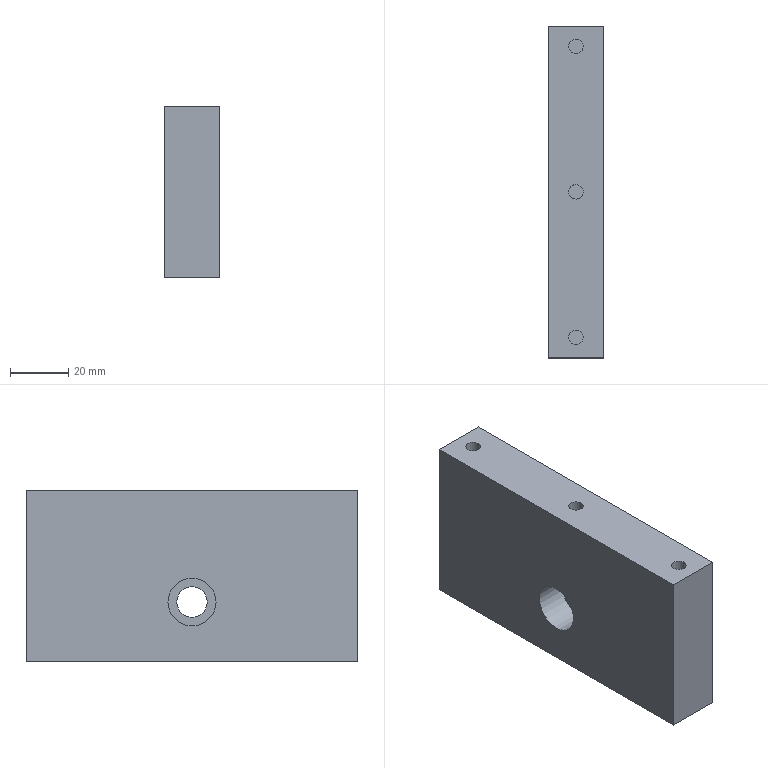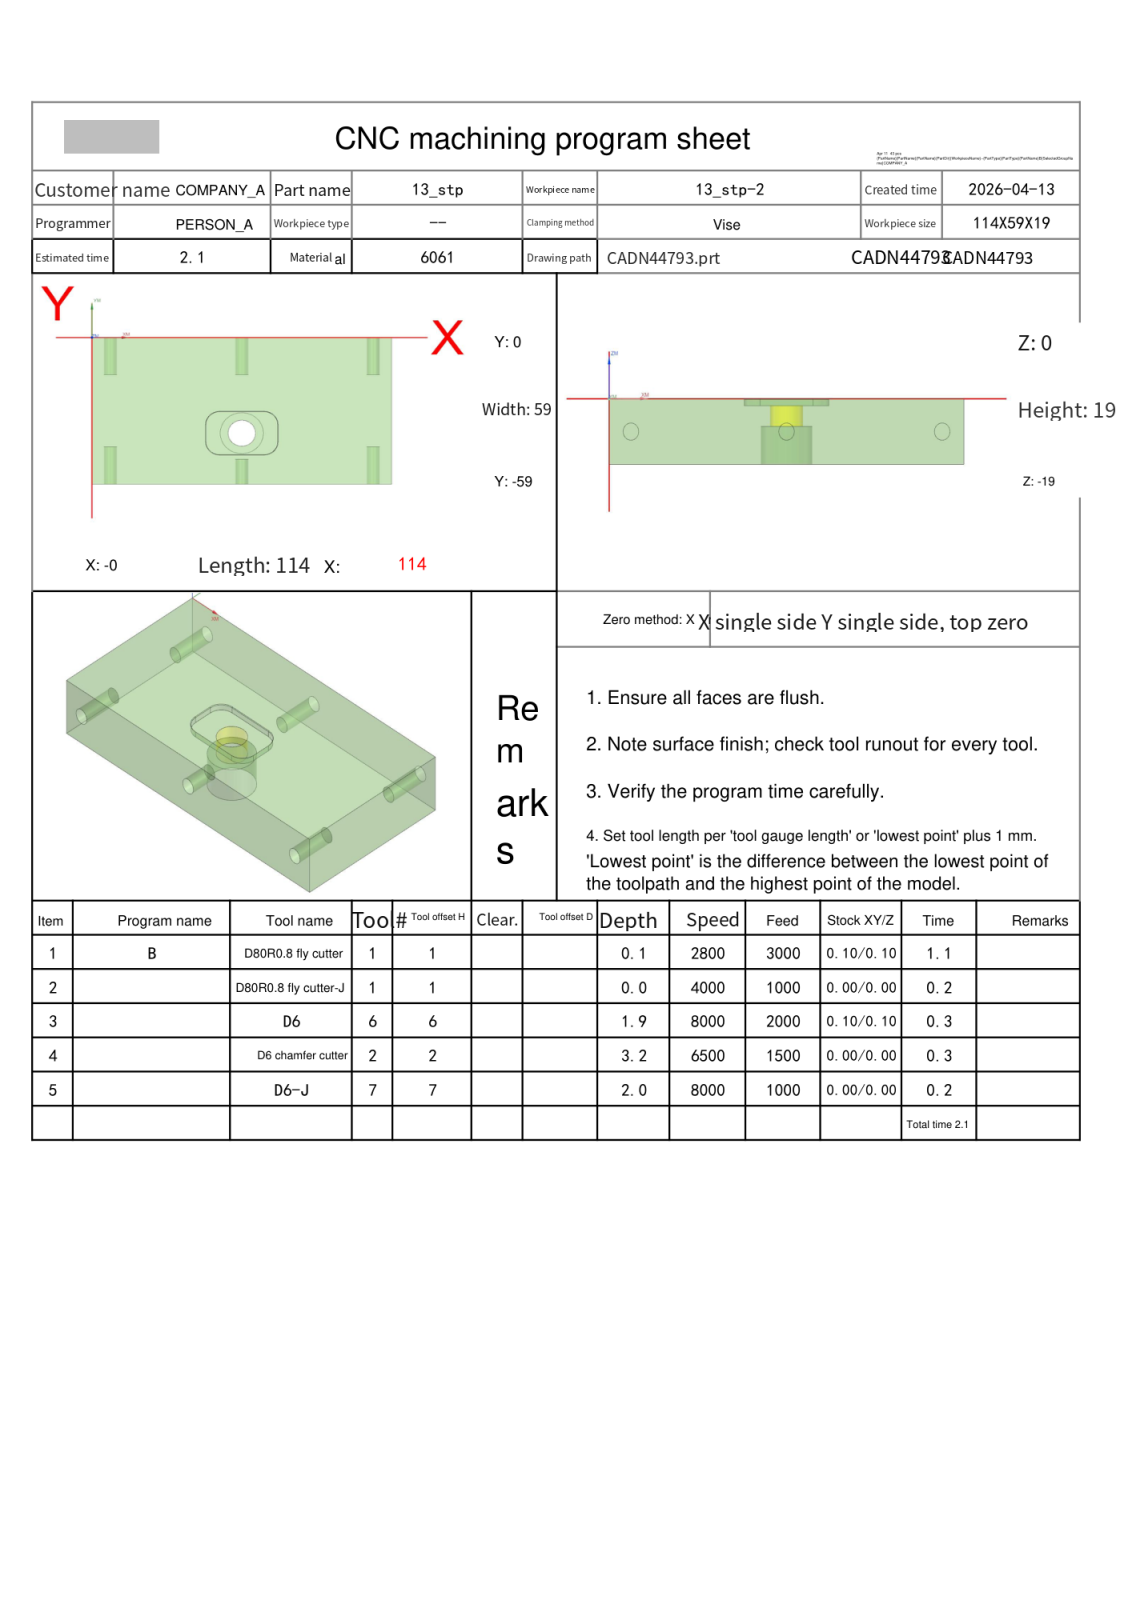NC program | NX | posted by the shop | part box 19 x 114 x 59 mm
Whole program:
%
O0001
(Machine time: 3.01 MIN)
(===Total Tool:4===)
(T1=D80R0.8 fly cutter D=80.  R=0.8  D- H01 Z=0.    )
(T6=D6      D=6.   R=0.   D-  H06 Z=-1.9  )
(T2=D6 chamfer cutter   D=6.   R=0.   D- H02 Z=-3.2  )
(T7=D6-J    D=6.   R=0.   D7  H07 Z=-2.   )
G80 G90 G17 G49 G40
G91 G28 Z0
M01
N1 T01 M06
(D80R0.8 fly cutter  D=80. R=0.8 H=01 ce=0.10 di=0.10)
G00 G90 G54 X-52.097 Y-29.5 M03 S2800
G43 H01 Z20.
M08
Z7.009
G01 Z5.009 F3000.
X-40.097
X154.097
X166.097
Z7.009
G00 X-52.097
Z6.518
G01 Z4.518
X-40.097
X154.097
X166.097
Z6.518
G00 X-52.097
Z6.027
G01 Z4.027
X-40.097
X154.097
X166.097
Z6.027
G00 X-52.097
Z5.536
G01 Z3.536
X-40.097
X154.097
X166.097
Z5.536
G00 Z20.
X-52.097
Z5.045
G01 Z3.045
X-40.097
X154.097
X166.097
Z5.045
G00 Z20.
X-52.097
Z4.555
G01 Z2.555
X-40.097
X154.097
X166.097
Z4.555
G00 Z20.
X-52.097
Z4.064
G01 Z2.064
X-40.097
X154.097
X166.097
Z4.064
G00 Z20.
X-52.097
Z3.573
G01 Z1.573
X-40.097
X154.097
X166.097
Z3.573
G00 Z20.
X-52.097
Z3.082
G01 Z1.082
X-40.097
X154.097
X166.097
Z3.082
G00 Z20.
X-52.097
Z2.591
G01 Z.591
X-40.097
X154.097
X166.097
Z2.591
G00 Z20.
X-52.097
Z2.1
G01 Z.1
X-40.097
X154.097
X166.097
Z2.1
G00 Z20.
G91 G28 Z0.0
M05
M09
G91 G28 Z0.0
M01
N2 T01 M06
(D80R0.8 fly cutter-J  D=80. R=0.8 H=01 ce=0.00 di=0.00)
G00 G90 G54 X-51.999 Y-29.5 M03 S4000
G43 H01 Z20.
M08
Z2.
G01 Z0.0 F1000.
X-39.999
X153.999
X165.999
Z2.
G00 Z20.
G91 G28 Z0.0
M05
M09
G91 G28 Z0.0
M01
N3 T06 M06
(D6  D=6. R=0. H=06 ce=0.10 di=0.10)
G00 G90 G54 X54.343 Y-37.233 M03 S8000
G43 H06 Z15.8
M08
Z1.5
G03 X54.343 Y-37.233 Z.611 I2.657 J.483 F2000.
X54.343 Y-37.233 Z-.278 I2.657 J.483
X57. Y-39.45 Z-.475 I2.657 J.483
G01 X62.401
G03 X63. Y-38.851 I-.001 J.6
G01 Y-38.049
G03 X62.401 Y-37.45 I-.6 J-.001
G01 X51.599
G03 X51. Y-38.049 I.001 J-.6
G01 Y-38.851
G03 X51.599 Y-39.45 I.6 J.001
G01 X55.179
G02 X55.678 Y-39.717 I0.0 J-.6
G01 X58.322 Y-43.683
G03 X58.821 Y-43.95 I.499 J.333
G01 X65.5
G03 X67.5 Y-41.95 I0.0 J2.
G01 Y-34.95
G03 X65.5 Y-32.95 I-2. J0.0
G01 X48.5
G03 X46.5 Y-34.95 I0.0 J-2.
G01 Y-41.95
G03 X48.5 Y-43.95 I2. J0.0
G01 X60.
X60.5
Y-40.95
Z1.025
G00 X54.343 Y-37.233
G03 X54.343 Y-37.233 Z.136 I2.657 J.483
X54.343 Y-37.233 Z-.753 I2.657 J.483
X57. Y-39.45 Z-.95 I2.657 J.483
G01 X62.401
G03 X63. Y-38.851 I-.001 J.6
G01 Y-38.049
G03 X62.401 Y-37.45 I-.6 J-.001
G01 X51.599
G03 X51. Y-38.049 I.001 J-.6
G01 Y-38.851
G03 X51.599 Y-39.45 I.6 J.001
G01 X55.179
G02 X55.678 Y-39.717 I0.0 J-.6
G01 X58.322 Y-43.683
G03 X58.821 Y-43.95 I.499 J.333
G01 X65.5
G03 X67.5 Y-41.95 I0.0 J2.
G01 Y-34.95
G03 X65.5 Y-32.95 I-2. J0.0
G01 X48.5
G03 X46.5 Y-34.95 I0.0 J-2.
G01 Y-41.95
G03 X48.5 Y-43.95 I2. J0.0
G01 X60.
X60.5
Y-40.95
Z.55
G00 X54.343 Y-37.233
G03 X54.343 Y-37.233 Z-.339 I2.657 J.483
X54.343 Y-37.233 Z-1.228 I2.657 J.483
X57. Y-39.45 Z-1.425 I2.657 J.483
G01 X62.401
G03 X63. Y-38.851 I-.001 J.6
G01 Y-38.049
G03 X62.401 Y-37.45 I-.6 J-.001
G01 X51.599
G03 X51. Y-38.049 I.001 J-.6
G01 Y-38.851
G03 X51.599 Y-39.45 I.6 J.001
G01 X55.179
G02 X55.678 Y-39.717 I0.0 J-.6
G01 X58.322 Y-43.683
G03 X58.821 Y-43.95 I.499 J.333
G01 X65.5
G03 X67.5 Y-41.95 I0.0 J2.
G01 Y-34.95
G03 X65.5 Y-32.95 I-2. J0.0
G01 X48.5
G03 X46.5 Y-34.95 I0.0 J-2.
G01 Y-41.95
G03 X48.5 Y-43.95 I2. J0.0
G01 X60.
X60.5
Y-40.95
Z.075
G00 X54.343 Y-37.233
G03 X54.343 Y-37.233 Z-.814 I2.657 J.483
X54.343 Y-37.233 Z-1.703 I2.657 J.483
X57. Y-39.45 Z-1.9 I2.657 J.483
G01 X62.401
G03 X63. Y-38.851 I-.001 J.6
G01 Y-38.049
G03 X62.401 Y-37.45 I-.6 J-.001
G01 X51.599
G03 X51. Y-38.049 I.001 J-.6
G01 Y-38.851
G03 X51.599 Y-39.45 I.6 J.001
G01 X55.179
G02 X55.678 Y-39.717 I0.0 J-.6
G01 X58.322 Y-43.683
G03 X58.821 Y-43.95 I.499 J.333
G01 X65.5
G03 X67.5 Y-41.95 I0.0 J2.
G01 Y-34.95
G03 X65.5 Y-32.95 I-2. J0.0
G01 X48.5
G03 X46.5 Y-34.95 I0.0 J-2.
G01 Y-41.95
G03 X48.5 Y-43.95 I2. J0.0
G01 X60.
X60.5
Y-40.95
Z-.4
G00 Z15.8
G91 G28 Z0.0
M05
M09
G91 G28 Z0.0
M01
N4 T02 M06
(D6 chamfer cutter  D=6. R=0. H=02 ce=0.00 di=0.00)
G00 G90 G54 X57.386 Y-60.227 M03 S6500
G43 H02 Z20.
M08
Z.172
G01 Z-1.2 F1500.
G03 X57.1 Y-60.027 I-1.286 J-1.532
G01 X57.054 Y-59.997
X57. Y-60.
X0.0
G02 X-1. Y-59. I0.0 J1.
G01 Y0.0
G02 X0.0 Y1. I1. J0.0
G01 X114.
G02 X115. Y0.0 I0.0 J-1.
G01 Y-59.
G02 X114. Y-60. I-1. J0.0
G01 X57.
X56.946 Y-59.997
X56.9 Y-60.027
G03 X56.614 Y-60.227 I1. J-1.732
G01 Z.172
G00 Z10.
X57.4 Y-34.401
Z-1.779
G01 Z-3.2
G03 X57.102 Y-34.22 I-1.183 J-1.613
G01 X57.054 Y-34.194
X57. Y-34.2
G03 X52.75 Y-38.45 I0.0 J-4.25
X57. Y-42.7 I4.25 J0.0
X61.25 Y-38.45 I0.0 J4.25
X57. Y-34.2 I-4.25 J0.0
G01 X56.946 Y-34.194
X56.898 Y-34.22
G03 X56.6 Y-34.401 I.885 J-1.794
G01 Z-1.773
G00 Z20.
G00 G90 X47.3 Y-44.916 M03 S6500
Z20.
Z.6
G01 Z-.9 F1500.
Y-45.15
G03 X48.5 Y-46.35 I1.2 J0.0
G01 X65.5
G03 X69.9 Y-41.95 I0.0 J4.4
G01 Y-34.95
G03 X65.5 Y-30.55 I-4.4 J0.0
G01 X48.5
G03 X44.1 Y-34.95 I0.0 J-4.4
G01 Y-41.95
G03 X48.5 Y-46.35 I4.4 J0.0
G01 X48.9
G03 X50.1 Y-45.15 I0.0 J1.2
G01 Z.6
G00 Z20.
G91 G28 Z0.0
M05
M09
G91 G28 Z0.0
M01
N5 T07 M06
(D6-J  D=6. R=0. H=07 ce=0.40 di=0.00)
G00 G90 G54 X64.2 Y-40.138 M03 S8000
G43 H07 Z15.8
M08
Z0.0
G01 Y-40.161 Z-.006 F1000.
X64.109 Y-40.387 Z-.071
X63.937 Y-40.559 Z-.137
X63.711 Y-40.65 Z-.202
X63.601 Z-.231
X57. Z-2.
Y-43.65
X48.5
G02 X46.8 Y-41.95 I0.0 J1.7
G01 Y-34.95
G02 X48.5 Y-33.25 I1.7 J0.0
G01 X65.5
G02 X67.2 Y-34.95 I0.0 J-1.7
G01 Y-41.95
G02 X65.5 Y-43.65 I-1.7 J0.0
G01 X55.748
G02 X55.324 Y-43.474 I0.0 J.6
G01 X52.676 Y-40.826
G03 X52.252 Y-40.65 I-.424 J-.424
G01 X50.399
G02 X49.8 Y-40.051 I.001 J.6
G01 Y-36.849
G02 X50.399 Y-36.25 I.6 J-.001
G01 X63.601
G02 X64.2 Y-36.849 I-.001 J-.6
G01 Y-40.051
G02 X63.601 Y-40.65 I-.6 J.001
G01 X54.
X53.
G03 X51.8 Y-41.85 I0.0 J-1.2
G01 Z-.5
G00 Z15.8
G00 G90 X47.78 Y-42.49 M03 S8000
Z15.8
Z-1.
G01 Z-2. F1000.
G41 D07
X47.3 Y-42.85
G03 X48.5 Y-44.05 I1.2 J0.0
G01 X65.5
G03 X67.6 Y-41.95 I0.0 J2.1
G01 Y-34.95
G03 X65.5 Y-32.85 I-2.1 J0.0
G01 X48.5
G03 X46.4 Y-34.95 I0.0 J-2.1
G01 Y-41.95
G03 X48.5 Y-44.05 I2.1 J0.0
G01 X48.9
G03 X50.1 Y-42.85 I0.0 J1.2
G01 G40 Y-42.65
Z-1.
G00 Z15.8
M05
M09
G91 G28 Z0.0
G91 G28 Y0.0
M30
%